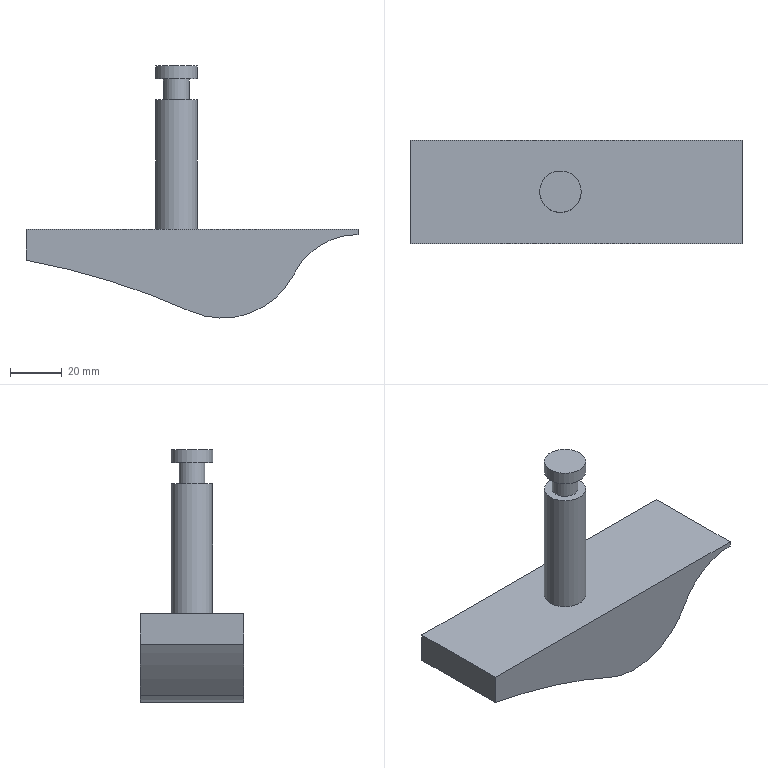Part | STEP file | tieqianhuakuai | 1 solid | 14 faces | box 128 x 40 x 97.212 mm | volume 118551 mm3 | plane 8 | cylinder 6 | commonest cylinder face diameters 16 x2 10 x1 55.183 x1 61.631 x1 558.782 x1
STEP:
#1=CARTESIAN_POINT('',(0.,0.,0.));
#2=DIRECTION('',(0.,0.,1.));
#3=DIRECTION('',(1.,0.,0.));
#4=AXIS2_PLACEMENT_3D('',#1,#2,#3);
#5=CARTESIAN_POINT('',(-8.116,0.,60.7));
#6=VERTEX_POINT('',#5);
#7=CARTESIAN_POINT('',(1.884,0.,60.7));
#8=VERTEX_POINT('',#7);
#9=CARTESIAN_POINT('',(-3.116,0.,60.7));
#10=DIRECTION('',(0.,0.,1.));
#11=DIRECTION('',(1.,0.,0.));
#12=AXIS2_PLACEMENT_3D('',#9,#10,#11);
#13=CIRCLE('',#12,5.);
#14=CARTESIAN_POINT('',(-3.116,0.,60.7));
#15=DIRECTION('',(0.,0.,-1.));
#16=DIRECTION('',(-1.,0.,0.));
#17=AXIS2_PLACEMENT_3D('',#14,#15,#16);
#18=CYLINDRICAL_SURFACE('',#17,5.);
#19=CARTESIAN_POINT('',(9.425,0.));
#20=DIRECTION('',(-1.,0.));
#21=VECTOR('',#20,1.);
#22=LINE('',#19,#21);
#23=(GEOMETRIC_REPRESENTATION_CONTEXT(2)PARAMETRIC_REPRESENTATION_CONTEXT()REPRESENTATION_CONTEXT('',''));
#24=DEFINITIONAL_REPRESENTATION('',(#22),#23);
#25=PCURVE('',#18,#24);
#26=CARTESIAN_POINT('',(-3.116,0.,60.7));
#27=DIRECTION('',(0.,0.,1.));
#28=DIRECTION('',(1.,0.,0.));
#29=AXIS2_PLACEMENT_3D('',#26,#27,#28);
#30=PLANE('',#29);
#31=CARTESIAN_POINT('',(0.,0.));
#32=DIRECTION('',(1.,0.));
#33=AXIS2_PLACEMENT_2D('',#31,#32);
#34=CIRCLE('',#33,5.);
#35=(GEOMETRIC_REPRESENTATION_CONTEXT(2)PARAMETRIC_REPRESENTATION_CONTEXT()REPRESENTATION_CONTEXT('',''));
#36=DEFINITIONAL_REPRESENTATION('',(#34),#35);
#37=PCURVE('',#30,#36);
#38=SURFACE_CURVE('',#13,(#25,#37),.PCURVE_S1.);
#39=EDGE_CURVE('',#6,#8,#38,.T.);
#40=ORIENTED_EDGE('',*,*,#39,.F.);
#41=CARTESIAN_POINT('',(-8.116,0.,52.7));
#42=VERTEX_POINT('',#41);
#43=CARTESIAN_POINT('',(-8.116,0.,60.7));
#44=CARTESIAN_POINT('',(-8.116,0.,52.7));
#45=B_SPLINE_CURVE_WITH_KNOTS('',1,(#43,#44),.UNSPECIFIED.,.F.,.F.,(2,2),(0.,8.),.PIECEWISE_BEZIER_KNOTS.);
#46=CARTESIAN_POINT('',(6.283,0.));
#47=DIRECTION('',(0.,1.));
#48=VECTOR('',#47,1.);
#49=LINE('',#46,#48);
#50=(GEOMETRIC_REPRESENTATION_CONTEXT(2)PARAMETRIC_REPRESENTATION_CONTEXT()REPRESENTATION_CONTEXT('',''));
#51=DEFINITIONAL_REPRESENTATION('',(#49),#50);
#52=PCURVE('',#18,#51);
#53=CARTESIAN_POINT('',(0.,0.));
#54=DIRECTION('',(0.,1.));
#55=VECTOR('',#54,1.);
#56=LINE('',#53,#55);
#57=(GEOMETRIC_REPRESENTATION_CONTEXT(2)PARAMETRIC_REPRESENTATION_CONTEXT()REPRESENTATION_CONTEXT('',''));
#58=DEFINITIONAL_REPRESENTATION('',(#56),#57);
#59=PCURVE('',#18,#58);
#60=SEAM_CURVE('',#45,(#52,#59),.PCURVE_S1.);
#61=EDGE_CURVE('',#6,#42,#60,.T.);
#62=ORIENTED_EDGE('',*,*,#61,.T.);
#63=CARTESIAN_POINT('',(-3.116,0.,52.7));
#64=DIRECTION('',(0.,0.,-1.));
#65=DIRECTION('',(-1.,0.,0.));
#66=AXIS2_PLACEMENT_3D('',#63,#64,#65);
#67=CIRCLE('',#66,5.);
#68=CARTESIAN_POINT('',(0.,8.));
#69=DIRECTION('',(1.,0.));
#70=VECTOR('',#69,1.);
#71=LINE('',#68,#70);
#72=(GEOMETRIC_REPRESENTATION_CONTEXT(2)PARAMETRIC_REPRESENTATION_CONTEXT()REPRESENTATION_CONTEXT('',''));
#73=DEFINITIONAL_REPRESENTATION('',(#71),#72);
#74=PCURVE('',#18,#73);
#75=CARTESIAN_POINT('',(-3.116,0.,52.7));
#76=DIRECTION('',(0.,0.,-1.));
#77=DIRECTION('',(-1.,0.,0.));
#78=AXIS2_PLACEMENT_3D('',#75,#76,#77);
#79=PLANE('',#78);
#80=CARTESIAN_POINT('',(0.,0.));
#81=DIRECTION('',(1.,0.));
#82=AXIS2_PLACEMENT_2D('',#80,#81);
#83=CIRCLE('',#82,5.);
#84=(GEOMETRIC_REPRESENTATION_CONTEXT(2)PARAMETRIC_REPRESENTATION_CONTEXT()REPRESENTATION_CONTEXT('',''));
#85=DEFINITIONAL_REPRESENTATION('',(#83),#84);
#86=PCURVE('',#79,#85);
#87=SURFACE_CURVE('',#67,(#74,#86),.PCURVE_S1.);
#88=EDGE_CURVE('',#42,#42,#87,.T.);
#89=ORIENTED_EDGE('',*,*,#88,.F.);
#90=ORIENTED_EDGE('',*,*,#61,.F.);
#91=CARTESIAN_POINT('',(-3.116,0.,60.7));
#92=DIRECTION('',(0.,0.,1.));
#93=DIRECTION('',(1.,0.,0.));
#94=AXIS2_PLACEMENT_3D('',#91,#92,#93);
#95=CIRCLE('',#94,5.);
#96=CARTESIAN_POINT('',(3.142,0.));
#97=DIRECTION('',(-1.,0.));
#98=VECTOR('',#97,1.);
#99=LINE('',#96,#98);
#100=(GEOMETRIC_REPRESENTATION_CONTEXT(2)PARAMETRIC_REPRESENTATION_CONTEXT()REPRESENTATION_CONTEXT('',''));
#101=DEFINITIONAL_REPRESENTATION('',(#99),#100);
#102=PCURVE('',#18,#101);
#103=CARTESIAN_POINT('',(0.,0.));
#104=DIRECTION('',(1.,0.));
#105=AXIS2_PLACEMENT_2D('',#103,#104);
#106=CIRCLE('',#105,5.);
#107=(GEOMETRIC_REPRESENTATION_CONTEXT(2)PARAMETRIC_REPRESENTATION_CONTEXT()REPRESENTATION_CONTEXT('',''));
#108=DEFINITIONAL_REPRESENTATION('',(#106),#107);
#109=PCURVE('',#30,#108);
#110=SURFACE_CURVE('',#95,(#102,#109),.PCURVE_S1.);
#111=EDGE_CURVE('',#8,#6,#110,.T.);
#112=ORIENTED_EDGE('',*,*,#111,.F.);
#113=EDGE_LOOP('',(#40,#62,#89,#90,#112));
#114=FACE_BOUND('',#113,.T.);
#115=ADVANCED_FACE('',(#114),#18,.T.);
#116=CARTESIAN_POINT('',(4.884,0.,60.7));
#117=VERTEX_POINT('',#116);
#118=CARTESIAN_POINT('',(-3.116,0.,60.7));
#119=DIRECTION('',(0.,0.,1.));
#120=DIRECTION('',(1.,0.,0.));
#121=AXIS2_PLACEMENT_3D('',#118,#119,#120);
#122=CIRCLE('',#121,8.);
#123=CARTESIAN_POINT('',(0.,0.));
#124=DIRECTION('',(1.,0.));
#125=AXIS2_PLACEMENT_2D('',#123,#124);
#126=CIRCLE('',#125,8.);
#127=(GEOMETRIC_REPRESENTATION_CONTEXT(2)PARAMETRIC_REPRESENTATION_CONTEXT()REPRESENTATION_CONTEXT('',''));
#128=DEFINITIONAL_REPRESENTATION('',(#126),#127);
#129=PCURVE('',#30,#128);
#130=CARTESIAN_POINT('',(-3.116,0.,65.7));
#131=DIRECTION('',(0.,0.,-1.));
#132=DIRECTION('',(-1.,0.,0.));
#133=AXIS2_PLACEMENT_3D('',#130,#131,#132);
#134=CYLINDRICAL_SURFACE('',#133,8.);
#135=CARTESIAN_POINT('',(9.425,5.));
#136=DIRECTION('',(-1.,0.));
#137=VECTOR('',#136,1.);
#138=LINE('',#135,#137);
#139=(GEOMETRIC_REPRESENTATION_CONTEXT(2)PARAMETRIC_REPRESENTATION_CONTEXT()REPRESENTATION_CONTEXT('',''));
#140=DEFINITIONAL_REPRESENTATION('',(#138),#139);
#141=PCURVE('',#134,#140);
#142=SURFACE_CURVE('',#122,(#129,#141),.PCURVE_S1.);
#143=EDGE_CURVE('',#117,#117,#142,.T.);
#144=ORIENTED_EDGE('',*,*,#143,.F.);
#145=EDGE_LOOP('',(#144));
#146=FACE_BOUND('',#145,.T.);
#147=ORIENTED_EDGE('',*,*,#111,.T.);
#148=ORIENTED_EDGE('',*,*,#39,.T.);
#149=EDGE_LOOP('',(#147,#148));
#150=FACE_BOUND('',#149,.T.);
#151=ADVANCED_FACE('',(#146,#150),#30,.F.);
#152=CARTESIAN_POINT('',(4.884,0.,65.7));
#153=VERTEX_POINT('',#152);
#154=CARTESIAN_POINT('',(-3.116,0.,65.7));
#155=DIRECTION('',(0.,0.,1.));
#156=DIRECTION('',(1.,0.,0.));
#157=AXIS2_PLACEMENT_3D('',#154,#155,#156);
#158=CIRCLE('',#157,8.);
#159=CARTESIAN_POINT('',(9.425,0.));
#160=DIRECTION('',(-1.,0.));
#161=VECTOR('',#160,1.);
#162=LINE('',#159,#161);
#163=(GEOMETRIC_REPRESENTATION_CONTEXT(2)PARAMETRIC_REPRESENTATION_CONTEXT()REPRESENTATION_CONTEXT('',''));
#164=DEFINITIONAL_REPRESENTATION('',(#162),#163);
#165=PCURVE('',#134,#164);
#166=CARTESIAN_POINT('',(-3.116,0.,65.7));
#167=DIRECTION('',(0.,0.,1.));
#168=DIRECTION('',(1.,0.,0.));
#169=AXIS2_PLACEMENT_3D('',#166,#167,#168);
#170=PLANE('',#169);
#171=CARTESIAN_POINT('',(0.,0.));
#172=DIRECTION('',(1.,0.));
#173=AXIS2_PLACEMENT_2D('',#171,#172);
#174=CIRCLE('',#173,8.);
#175=(GEOMETRIC_REPRESENTATION_CONTEXT(2)PARAMETRIC_REPRESENTATION_CONTEXT()REPRESENTATION_CONTEXT('',''));
#176=DEFINITIONAL_REPRESENTATION('',(#174),#175);
#177=PCURVE('',#170,#176);
#178=SURFACE_CURVE('',#158,(#165,#177),.PCURVE_S1.);
#179=EDGE_CURVE('',#153,#153,#178,.T.);
#180=ORIENTED_EDGE('',*,*,#179,.F.);
#181=CARTESIAN_POINT('',(4.884,0.,65.7));
#182=CARTESIAN_POINT('',(4.884,0.,60.7));
#183=B_SPLINE_CURVE_WITH_KNOTS('',1,(#181,#182),.UNSPECIFIED.,.F.,.F.,(2,2),(0.,5.),.PIECEWISE_BEZIER_KNOTS.);
#184=CARTESIAN_POINT('',(9.425,0.));
#185=DIRECTION('',(0.,1.));
#186=VECTOR('',#185,1.);
#187=LINE('',#184,#186);
#188=(GEOMETRIC_REPRESENTATION_CONTEXT(2)PARAMETRIC_REPRESENTATION_CONTEXT()REPRESENTATION_CONTEXT('',''));
#189=DEFINITIONAL_REPRESENTATION('',(#187),#188);
#190=PCURVE('',#134,#189);
#191=CARTESIAN_POINT('',(3.142,0.));
#192=DIRECTION('',(0.,1.));
#193=VECTOR('',#192,1.);
#194=LINE('',#191,#193);
#195=(GEOMETRIC_REPRESENTATION_CONTEXT(2)PARAMETRIC_REPRESENTATION_CONTEXT()REPRESENTATION_CONTEXT('',''));
#196=DEFINITIONAL_REPRESENTATION('',(#194),#195);
#197=PCURVE('',#134,#196);
#198=SEAM_CURVE('',#183,(#190,#197),.PCURVE_S1.);
#199=EDGE_CURVE('',#153,#117,#198,.T.);
#200=ORIENTED_EDGE('',*,*,#199,.T.);
#201=ORIENTED_EDGE('',*,*,#143,.T.);
#202=ORIENTED_EDGE('',*,*,#199,.F.);
#203=EDGE_LOOP('',(#180,#200,#201,#202));
#204=FACE_BOUND('',#203,.T.);
#205=ADVANCED_FACE('',(#204),#134,.T.);
#206=ORIENTED_EDGE('',*,*,#179,.T.);
#207=EDGE_LOOP('',(#206));
#208=FACE_BOUND('',#207,.T.);
#209=ADVANCED_FACE('',(#208),#170,.T.);
#210=CARTESIAN_POINT('',(-11.116,0.,52.7));
#211=VERTEX_POINT('',#210);
#212=CARTESIAN_POINT('',(-3.116,0.,52.7));
#213=DIRECTION('',(0.,0.,-1.));
#214=DIRECTION('',(-1.,0.,0.));
#215=AXIS2_PLACEMENT_3D('',#212,#213,#214);
#216=CIRCLE('',#215,8.);
#217=CARTESIAN_POINT('',(0.,0.));
#218=DIRECTION('',(1.,0.));
#219=AXIS2_PLACEMENT_2D('',#217,#218);
#220=CIRCLE('',#219,8.);
#221=(GEOMETRIC_REPRESENTATION_CONTEXT(2)PARAMETRIC_REPRESENTATION_CONTEXT()REPRESENTATION_CONTEXT('',''));
#222=DEFINITIONAL_REPRESENTATION('',(#220),#221);
#223=PCURVE('',#79,#222);
#224=CARTESIAN_POINT('',(-3.116,0.,2.7));
#225=DIRECTION('',(0.,0.,1.));
#226=DIRECTION('',(1.,0.,0.));
#227=AXIS2_PLACEMENT_3D('',#224,#225,#226);
#228=CYLINDRICAL_SURFACE('',#227,8.);
#229=CARTESIAN_POINT('',(9.425,50.));
#230=DIRECTION('',(-1.,0.));
#231=VECTOR('',#230,1.);
#232=LINE('',#229,#231);
#233=(GEOMETRIC_REPRESENTATION_CONTEXT(2)PARAMETRIC_REPRESENTATION_CONTEXT()REPRESENTATION_CONTEXT('',''));
#234=DEFINITIONAL_REPRESENTATION('',(#232),#233);
#235=PCURVE('',#228,#234);
#236=SURFACE_CURVE('',#216,(#223,#235),.PCURVE_S1.);
#237=EDGE_CURVE('',#211,#211,#236,.T.);
#238=ORIENTED_EDGE('',*,*,#237,.F.);
#239=EDGE_LOOP('',(#238));
#240=FACE_BOUND('',#239,.T.);
#241=ORIENTED_EDGE('',*,*,#88,.T.);
#242=EDGE_LOOP('',(#241));
#243=FACE_BOUND('',#242,.T.);
#244=ADVANCED_FACE('',(#240,#243),#79,.F.);
#245=CARTESIAN_POINT('',(-11.116,0.,2.7));
#246=VERTEX_POINT('',#245);
#247=CARTESIAN_POINT('',(-3.116,0.,2.7));
#248=DIRECTION('',(0.,0.,-1.));
#249=DIRECTION('',(-1.,0.,0.));
#250=AXIS2_PLACEMENT_3D('',#247,#248,#249);
#251=CIRCLE('',#250,8.);
#252=CARTESIAN_POINT('',(9.425,0.));
#253=DIRECTION('',(-1.,0.));
#254=VECTOR('',#253,1.);
#255=LINE('',#252,#254);
#256=(GEOMETRIC_REPRESENTATION_CONTEXT(2)PARAMETRIC_REPRESENTATION_CONTEXT()REPRESENTATION_CONTEXT('',''));
#257=DEFINITIONAL_REPRESENTATION('',(#255),#256);
#258=PCURVE('',#228,#257);
#259=CARTESIAN_POINT('',(-61.116,-20.,2.7));
#260=DIRECTION('',(0.,0.,1.));
#261=DIRECTION('',(1.,0.,0.));
#262=AXIS2_PLACEMENT_3D('',#259,#260,#261);
#263=PLANE('',#262);
#264=CARTESIAN_POINT('',(50.,20.));
#265=CARTESIAN_POINT('',(50.,33.856));
#266=CARTESIAN_POINT('',(62.,26.928));
#267=CARTESIAN_POINT('',(74.,20.));
#268=CARTESIAN_POINT('',(62.,13.072));
#269=CARTESIAN_POINT('',(50.,6.144));
#270=CARTESIAN_POINT('',(50.,20.));
#271=(BOUNDED_CURVE()B_SPLINE_CURVE(2,(#264,#265,#266,#267,#268,#269,#270),.UNSPECIFIED.,.T.,.F.)B_SPLINE_CURVE_WITH_KNOTS((1,2,2,2,2,1),(-2.094,0.,2.094,4.189,6.283,8.378),.UNSPECIFIED.)CURVE()GEOMETRIC_REPRESENTATION_ITEM()RATIONAL_B_SPLINE_CURVE((1.,0.5,1.,0.5,1.,0.5,1.))REPRESENTATION_ITEM(''));
#272=(GEOMETRIC_REPRESENTATION_CONTEXT(2)PARAMETRIC_REPRESENTATION_CONTEXT()REPRESENTATION_CONTEXT('',''));
#273=DEFINITIONAL_REPRESENTATION('',(#271),#272);
#274=PCURVE('',#263,#273);
#275=SURFACE_CURVE('',#251,(#258,#274),.PCURVE_S1.);
#276=EDGE_CURVE('',#246,#246,#275,.T.);
#277=ORIENTED_EDGE('',*,*,#276,.F.);
#278=CARTESIAN_POINT('',(-11.116,0.,2.7));
#279=CARTESIAN_POINT('',(-11.116,0.,52.7));
#280=B_SPLINE_CURVE_WITH_KNOTS('',1,(#278,#279),.UNSPECIFIED.,.F.,.F.,(2,2),(0.,50.),.PIECEWISE_BEZIER_KNOTS.);
#281=CARTESIAN_POINT('',(9.425,0.));
#282=DIRECTION('',(0.,1.));
#283=VECTOR('',#282,1.);
#284=LINE('',#281,#283);
#285=(GEOMETRIC_REPRESENTATION_CONTEXT(2)PARAMETRIC_REPRESENTATION_CONTEXT()REPRESENTATION_CONTEXT('',''));
#286=DEFINITIONAL_REPRESENTATION('',(#284),#285);
#287=PCURVE('',#228,#286);
#288=CARTESIAN_POINT('',(3.142,0.));
#289=DIRECTION('',(0.,1.));
#290=VECTOR('',#289,1.);
#291=LINE('',#288,#290);
#292=(GEOMETRIC_REPRESENTATION_CONTEXT(2)PARAMETRIC_REPRESENTATION_CONTEXT()REPRESENTATION_CONTEXT('',''));
#293=DEFINITIONAL_REPRESENTATION('',(#291),#292);
#294=PCURVE('',#228,#293);
#295=SEAM_CURVE('',#280,(#287,#294),.PCURVE_S1.);
#296=EDGE_CURVE('',#246,#211,#295,.T.);
#297=ORIENTED_EDGE('',*,*,#296,.T.);
#298=ORIENTED_EDGE('',*,*,#237,.T.);
#299=ORIENTED_EDGE('',*,*,#296,.F.);
#300=EDGE_LOOP('',(#277,#297,#298,#299));
#301=FACE_BOUND('',#300,.T.);
#302=ADVANCED_FACE('',(#301),#228,.T.);
#303=CARTESIAN_POINT('',(66.884,-20.,2.7));
#304=VERTEX_POINT('',#303);
#305=CARTESIAN_POINT('',(66.884,20.,2.7));
#306=VERTEX_POINT('',#305);
#307=CARTESIAN_POINT('',(66.884,-20.,2.7));
#308=DIRECTION('',(0.,1.,0.));
#309=VECTOR('',#308,1.);
#310=LINE('',#307,#309);
#311=CARTESIAN_POINT('',(128.,0.));
#312=DIRECTION('',(0.,1.));
#313=VECTOR('',#312,1.);
#314=LINE('',#311,#313);
#315=(GEOMETRIC_REPRESENTATION_CONTEXT(2)PARAMETRIC_REPRESENTATION_CONTEXT()REPRESENTATION_CONTEXT('',''));
#316=DEFINITIONAL_REPRESENTATION('',(#314),#315);
#317=PCURVE('',#263,#316);
#318=CARTESIAN_POINT('',(66.884,-20.,2.7));
#319=DIRECTION('',(1.,0.,0.));
#320=DIRECTION('',(0.,0.,-1.));
#321=AXIS2_PLACEMENT_3D('',#318,#319,#320);
#322=PLANE('',#321);
#323=CARTESIAN_POINT('',(0.,0.));
#324=DIRECTION('',(0.,1.));
#325=VECTOR('',#324,1.);
#326=LINE('',#323,#325);
#327=(GEOMETRIC_REPRESENTATION_CONTEXT(2)PARAMETRIC_REPRESENTATION_CONTEXT()REPRESENTATION_CONTEXT('',''));
#328=DEFINITIONAL_REPRESENTATION('',(#326),#327);
#329=PCURVE('',#322,#328);
#330=SURFACE_CURVE('',#310,(#317,#329),.PCURVE_S1.);
#331=EDGE_CURVE('',#304,#306,#330,.T.);
#332=ORIENTED_EDGE('',*,*,#331,.T.);
#333=CARTESIAN_POINT('',(-61.116,20.,2.7));
#334=VERTEX_POINT('',#333);
#335=CARTESIAN_POINT('',(-11.116,20.,2.7));
#336=DIRECTION('',(1.,0.,0.));
#337=VECTOR('',#336,1.);
#338=LINE('',#335,#337);
#339=CARTESIAN_POINT('',(50.,40.));
#340=DIRECTION('',(1.,0.));
#341=VECTOR('',#340,1.);
#342=LINE('',#339,#341);
#343=(GEOMETRIC_REPRESENTATION_CONTEXT(2)PARAMETRIC_REPRESENTATION_CONTEXT()REPRESENTATION_CONTEXT('',''));
#344=DEFINITIONAL_REPRESENTATION('',(#342),#343);
#345=PCURVE('',#263,#344);
#346=CARTESIAN_POINT('',(66.884,20.,-26.891));
#347=DIRECTION('',(0.,-1.,0.));
#348=DIRECTION('',(0.,0.,-1.));
#349=AXIS2_PLACEMENT_3D('',#346,#347,#348);
#350=PLANE('',#349);
#351=CARTESIAN_POINT('',(-29.592,-78.));
#352=DIRECTION('',(0.,1.));
#353=VECTOR('',#352,1.);
#354=LINE('',#351,#353);
#355=(GEOMETRIC_REPRESENTATION_CONTEXT(2)PARAMETRIC_REPRESENTATION_CONTEXT()REPRESENTATION_CONTEXT('',''));
#356=DEFINITIONAL_REPRESENTATION('',(#354),#355);
#357=PCURVE('',#350,#356);
#358=SURFACE_CURVE('',#338,(#345,#357),.PCURVE_S1.);
#359=EDGE_CURVE('',#334,#306,#358,.T.);
#360=ORIENTED_EDGE('',*,*,#359,.F.);
#361=CARTESIAN_POINT('',(-61.116,-20.,2.7));
#362=VERTEX_POINT('',#361);
#363=CARTESIAN_POINT('',(-61.116,-20.,2.7));
#364=DIRECTION('',(0.,1.,0.));
#365=VECTOR('',#364,1.);
#366=LINE('',#363,#365);
#367=CARTESIAN_POINT('',(0.,0.));
#368=DIRECTION('',(0.,1.));
#369=VECTOR('',#368,1.);
#370=LINE('',#367,#369);
#371=(GEOMETRIC_REPRESENTATION_CONTEXT(2)PARAMETRIC_REPRESENTATION_CONTEXT()REPRESENTATION_CONTEXT('',''));
#372=DEFINITIONAL_REPRESENTATION('',(#370),#371);
#373=PCURVE('',#263,#372);
#374=CARTESIAN_POINT('',(-61.116,-20.,-9.241));
#375=DIRECTION('',(-1.,0.,0.));
#376=DIRECTION('',(0.,0.,1.));
#377=AXIS2_PLACEMENT_3D('',#374,#375,#376);
#378=PLANE('',#377);
#379=CARTESIAN_POINT('',(11.941,0.));
#380=DIRECTION('',(0.,1.));
#381=VECTOR('',#380,1.);
#382=LINE('',#379,#381);
#383=(GEOMETRIC_REPRESENTATION_CONTEXT(2)PARAMETRIC_REPRESENTATION_CONTEXT()REPRESENTATION_CONTEXT('',''));
#384=DEFINITIONAL_REPRESENTATION('',(#382),#383);
#385=PCURVE('',#378,#384);
#386=SURFACE_CURVE('',#366,(#373,#385),.PCURVE_S1.);
#387=EDGE_CURVE('',#362,#334,#386,.T.);
#388=ORIENTED_EDGE('',*,*,#387,.F.);
#389=CARTESIAN_POINT('',(-11.116,-20.,2.7));
#390=DIRECTION('',(1.,0.,0.));
#391=VECTOR('',#390,1.);
#392=LINE('',#389,#391);
#393=CARTESIAN_POINT('',(50.,0.));
#394=DIRECTION('',(1.,0.));
#395=VECTOR('',#394,1.);
#396=LINE('',#393,#395);
#397=(GEOMETRIC_REPRESENTATION_CONTEXT(2)PARAMETRIC_REPRESENTATION_CONTEXT()REPRESENTATION_CONTEXT('',''));
#398=DEFINITIONAL_REPRESENTATION('',(#396),#397);
#399=PCURVE('',#263,#398);
#400=CARTESIAN_POINT('',(66.884,-20.,-26.891));
#401=DIRECTION('',(0.,-1.,0.));
#402=DIRECTION('',(0.,0.,-1.));
#403=AXIS2_PLACEMENT_3D('',#400,#401,#402);
#404=PLANE('',#403);
#405=CARTESIAN_POINT('',(-29.592,-78.));
#406=DIRECTION('',(0.,1.));
#407=VECTOR('',#406,1.);
#408=LINE('',#405,#407);
#409=(GEOMETRIC_REPRESENTATION_CONTEXT(2)PARAMETRIC_REPRESENTATION_CONTEXT()REPRESENTATION_CONTEXT('',''));
#410=DEFINITIONAL_REPRESENTATION('',(#408),#409);
#411=PCURVE('',#404,#410);
#412=SURFACE_CURVE('',#392,(#399,#411),.PCURVE_S1.);
#413=EDGE_CURVE('',#362,#304,#412,.T.);
#414=ORIENTED_EDGE('',*,*,#413,.T.);
#415=EDGE_LOOP('',(#332,#360,#388,#414));
#416=FACE_BOUND('',#415,.T.);
#417=ORIENTED_EDGE('',*,*,#276,.T.);
#418=EDGE_LOOP('',(#417));
#419=FACE_BOUND('',#418,.T.);
#420=ADVANCED_FACE('',(#416,#419),#263,.T.);
#421=ORIENTED_EDGE('',*,*,#387,.T.);
#422=CARTESIAN_POINT('',(-61.116,20.,-9.241));
#423=VERTEX_POINT('',#422);
#424=CARTESIAN_POINT('',(-61.116,20.,-9.241));
#425=DIRECTION('',(0.,0.,1.));
#426=VECTOR('',#425,1.);
#427=LINE('',#424,#426);
#428=CARTESIAN_POINT('',(0.,40.));
#429=DIRECTION('',(1.,0.));
#430=VECTOR('',#429,1.);
#431=LINE('',#428,#430);
#432=(GEOMETRIC_REPRESENTATION_CONTEXT(2)PARAMETRIC_REPRESENTATION_CONTEXT()REPRESENTATION_CONTEXT('',''));
#433=DEFINITIONAL_REPRESENTATION('',(#431),#432);
#434=PCURVE('',#378,#433);
#435=CARTESIAN_POINT('',(-17.65,-128.));
#436=DIRECTION('',(-1.,0.));
#437=VECTOR('',#436,1.);
#438=LINE('',#435,#437);
#439=(GEOMETRIC_REPRESENTATION_CONTEXT(2)PARAMETRIC_REPRESENTATION_CONTEXT()REPRESENTATION_CONTEXT('',''));
#440=DEFINITIONAL_REPRESENTATION('',(#438),#439);
#441=PCURVE('',#350,#440);
#442=SURFACE_CURVE('',#427,(#434,#441),.PCURVE_S1.);
#443=EDGE_CURVE('',#423,#334,#442,.T.);
#444=ORIENTED_EDGE('',*,*,#443,.F.);
#445=CARTESIAN_POINT('',(-61.116,-20.,-9.241));
#446=VERTEX_POINT('',#445);
#447=CARTESIAN_POINT('',(-61.116,-20.,-9.241));
#448=DIRECTION('',(0.,1.,0.));
#449=VECTOR('',#448,1.);
#450=LINE('',#447,#449);
#451=CARTESIAN_POINT('',(0.,0.));
#452=DIRECTION('',(0.,1.));
#453=VECTOR('',#452,1.);
#454=LINE('',#451,#453);
#455=(GEOMETRIC_REPRESENTATION_CONTEXT(2)PARAMETRIC_REPRESENTATION_CONTEXT()REPRESENTATION_CONTEXT('',''));
#456=DEFINITIONAL_REPRESENTATION('',(#454),#455);
#457=PCURVE('',#378,#456);
#458=CARTESIAN_POINT('',(-111.608,-20.,-284.032));
#459=DIRECTION('',(0.,1.,0.));
#460=DIRECTION('',(0.,0.,1.));
#461=AXIS2_PLACEMENT_3D('',#458,#459,#460);
#462=CYLINDRICAL_SURFACE('',#461,279.391);
#463=CARTESIAN_POINT('',(0.1817,0.));
#464=DIRECTION('',(0.,1.));
#465=VECTOR('',#464,1.);
#466=LINE('',#463,#465);
#467=(GEOMETRIC_REPRESENTATION_CONTEXT(2)PARAMETRIC_REPRESENTATION_CONTEXT()REPRESENTATION_CONTEXT('',''));
#468=DEFINITIONAL_REPRESENTATION('',(#466),#467);
#469=PCURVE('',#462,#468);
#470=SURFACE_CURVE('',#450,(#457,#469),.PCURVE_S1.);
#471=EDGE_CURVE('',#446,#423,#470,.T.);
#472=ORIENTED_EDGE('',*,*,#471,.F.);
#473=CARTESIAN_POINT('',(-61.116,-20.,-9.241));
#474=DIRECTION('',(0.,0.,1.));
#475=VECTOR('',#474,1.);
#476=LINE('',#473,#475);
#477=CARTESIAN_POINT('',(0.,0.));
#478=DIRECTION('',(1.,0.));
#479=VECTOR('',#478,1.);
#480=LINE('',#477,#479);
#481=(GEOMETRIC_REPRESENTATION_CONTEXT(2)PARAMETRIC_REPRESENTATION_CONTEXT()REPRESENTATION_CONTEXT('',''));
#482=DEFINITIONAL_REPRESENTATION('',(#480),#481);
#483=PCURVE('',#378,#482);
#484=CARTESIAN_POINT('',(-17.65,-128.));
#485=DIRECTION('',(-1.,0.));
#486=VECTOR('',#485,1.);
#487=LINE('',#484,#486);
#488=(GEOMETRIC_REPRESENTATION_CONTEXT(2)PARAMETRIC_REPRESENTATION_CONTEXT()REPRESENTATION_CONTEXT('',''));
#489=DEFINITIONAL_REPRESENTATION('',(#487),#488);
#490=PCURVE('',#404,#489);
#491=SURFACE_CURVE('',#476,(#483,#490),.PCURVE_S1.);
#492=EDGE_CURVE('',#446,#362,#491,.T.);
#493=ORIENTED_EDGE('',*,*,#492,.T.);
#494=EDGE_LOOP('',(#421,#444,#472,#493));
#495=FACE_BOUND('',#494,.T.);
#496=ADVANCED_FACE('',(#495),#378,.T.);
#497=CARTESIAN_POINT('',(2.135,-20.,-28.842));
#498=VERTEX_POINT('',#497);
#499=CARTESIAN_POINT('',(-111.608,-20.,-284.032));
#500=DIRECTION('',(0.,-1.,0.));
#501=DIRECTION('',(0.,0.,-1.));
#502=AXIS2_PLACEMENT_3D('',#499,#500,#501);
#503=CIRCLE('',#502,279.391);
#504=CARTESIAN_POINT('',(3.142,0.));
#505=DIRECTION('',(-1.,0.));
#506=VECTOR('',#505,1.);
#507=LINE('',#504,#506);
#508=(GEOMETRIC_REPRESENTATION_CONTEXT(2)PARAMETRIC_REPRESENTATION_CONTEXT()REPRESENTATION_CONTEXT('',''));
#509=DEFINITIONAL_REPRESENTATION('',(#507),#508);
#510=PCURVE('',#462,#509);
#511=CARTESIAN_POINT('',(257.141,-178.492));
#512=DIRECTION('',(1.,0.));
#513=AXIS2_PLACEMENT_2D('',#511,#512);
#514=CIRCLE('',#513,279.391);
#515=(GEOMETRIC_REPRESENTATION_CONTEXT(2)PARAMETRIC_REPRESENTATION_CONTEXT()REPRESENTATION_CONTEXT('',''));
#516=DEFINITIONAL_REPRESENTATION('',(#514),#515);
#517=PCURVE('',#404,#516);
#518=SURFACE_CURVE('',#503,(#510,#517),.PCURVE_S1.);
#519=EDGE_CURVE('',#498,#446,#518,.T.);
#520=ORIENTED_EDGE('',*,*,#519,.F.);
#521=CARTESIAN_POINT('',(2.135,20.,-28.842));
#522=VERTEX_POINT('',#521);
#523=CARTESIAN_POINT('',(2.135,-20.,-28.842));
#524=DIRECTION('',(0.,1.,0.));
#525=VECTOR('',#524,1.);
#526=LINE('',#523,#525);
#527=CARTESIAN_POINT('',(0.4193,0.));
#528=DIRECTION('',(0.,1.));
#529=VECTOR('',#528,1.);
#530=LINE('',#527,#529);
#531=(GEOMETRIC_REPRESENTATION_CONTEXT(2)PARAMETRIC_REPRESENTATION_CONTEXT()REPRESENTATION_CONTEXT('',''));
#532=DEFINITIONAL_REPRESENTATION('',(#530),#531);
#533=PCURVE('',#462,#532);
#534=CARTESIAN_POINT('',(14.68,-20.,-0.6956));
#535=DIRECTION('',(0.,1.,0.));
#536=DIRECTION('',(0.,0.,1.));
#537=AXIS2_PLACEMENT_3D('',#534,#535,#536);
#538=CYLINDRICAL_SURFACE('',#537,30.816);
#539=CARTESIAN_POINT('',(3.561,0.));
#540=DIRECTION('',(0.,1.));
#541=VECTOR('',#540,1.);
#542=LINE('',#539,#541);
#543=(GEOMETRIC_REPRESENTATION_CONTEXT(2)PARAMETRIC_REPRESENTATION_CONTEXT()REPRESENTATION_CONTEXT('',''));
#544=DEFINITIONAL_REPRESENTATION('',(#542),#543);
#545=PCURVE('',#538,#544);
#546=SURFACE_CURVE('',#526,(#533,#545),.PCURVE_S1.);
#547=EDGE_CURVE('',#498,#522,#546,.T.);
#548=ORIENTED_EDGE('',*,*,#547,.T.);
#549=CARTESIAN_POINT('',(-111.608,20.,-284.032));
#550=DIRECTION('',(0.,-1.,0.));
#551=DIRECTION('',(0.,0.,-1.));
#552=AXIS2_PLACEMENT_3D('',#549,#550,#551);
#553=CIRCLE('',#552,279.391);
#554=CARTESIAN_POINT('',(3.142,40.));
#555=DIRECTION('',(-1.,0.));
#556=VECTOR('',#555,1.);
#557=LINE('',#554,#556);
#558=(GEOMETRIC_REPRESENTATION_CONTEXT(2)PARAMETRIC_REPRESENTATION_CONTEXT()REPRESENTATION_CONTEXT('',''));
#559=DEFINITIONAL_REPRESENTATION('',(#557),#558);
#560=PCURVE('',#462,#559);
#561=CARTESIAN_POINT('',(257.141,-178.492));
#562=DIRECTION('',(1.,0.));
#563=AXIS2_PLACEMENT_2D('',#561,#562);
#564=CIRCLE('',#563,279.391);
#565=(GEOMETRIC_REPRESENTATION_CONTEXT(2)PARAMETRIC_REPRESENTATION_CONTEXT()REPRESENTATION_CONTEXT('',''));
#566=DEFINITIONAL_REPRESENTATION('',(#564),#565);
#567=PCURVE('',#350,#566);
#568=SURFACE_CURVE('',#553,(#560,#567),.PCURVE_S1.);
#569=EDGE_CURVE('',#522,#423,#568,.T.);
#570=ORIENTED_EDGE('',*,*,#569,.T.);
#571=ORIENTED_EDGE('',*,*,#471,.F.);
#572=EDGE_LOOP('',(#520,#548,#570,#571));
#573=FACE_BOUND('',#572,.F.);
#574=ADVANCED_FACE('',(#573),#462,.F.);
#575=ORIENTED_EDGE('',*,*,#547,.T.);
#576=CARTESIAN_POINT('',(42.223,20.,-14.516));
#577=VERTEX_POINT('',#576);
#578=CARTESIAN_POINT('',(14.68,20.,-0.6956));
#579=DIRECTION('',(0.,1.,0.));
#580=DIRECTION('',(0.,0.,1.));
#581=AXIS2_PLACEMENT_3D('',#578,#579,#580);
#582=CIRCLE('',#581,30.816);
#583=CARTESIAN_POINT('',(0.,40.));
#584=DIRECTION('',(1.,0.));
#585=VECTOR('',#584,1.);
#586=LINE('',#583,#585);
#587=(GEOMETRIC_REPRESENTATION_CONTEXT(2)PARAMETRIC_REPRESENTATION_CONTEXT()REPRESENTATION_CONTEXT('',''));
#588=DEFINITIONAL_REPRESENTATION('',(#586),#587);
#589=PCURVE('',#538,#588);
#590=CARTESIAN_POINT('',(-57.011,-52.203));
#591=CARTESIAN_POINT('',(-57.011,1.171));
#592=CARTESIAN_POINT('',(-10.788,-25.516));
#593=CARTESIAN_POINT('',(35.436,-52.203));
#594=CARTESIAN_POINT('',(-10.788,-78.891));
#595=CARTESIAN_POINT('',(-57.011,-105.578));
#596=CARTESIAN_POINT('',(-57.011,-52.203));
#597=(BOUNDED_CURVE()B_SPLINE_CURVE(2,(#590,#591,#592,#593,#594,#595,#596),.UNSPECIFIED.,.T.,.F.)B_SPLINE_CURVE_WITH_KNOTS((1,2,2,2,2,1),(-2.094,0.,2.094,4.189,6.283,8.378),.UNSPECIFIED.)CURVE()GEOMETRIC_REPRESENTATION_ITEM()RATIONAL_B_SPLINE_CURVE((1.,0.5,1.,0.5,1.,0.5,1.))REPRESENTATION_ITEM(''));
#598=(GEOMETRIC_REPRESENTATION_CONTEXT(2)PARAMETRIC_REPRESENTATION_CONTEXT()REPRESENTATION_CONTEXT('',''));
#599=DEFINITIONAL_REPRESENTATION('',(#597),#598);
#600=PCURVE('',#350,#599);
#601=SURFACE_CURVE('',#582,(#589,#600),.PCURVE_S1.);
#602=EDGE_CURVE('',#577,#522,#601,.T.);
#603=ORIENTED_EDGE('',*,*,#602,.F.);
#604=CARTESIAN_POINT('',(42.223,-20.,-14.516));
#605=VERTEX_POINT('',#604);
#606=CARTESIAN_POINT('',(42.223,-20.,-14.516));
#607=DIRECTION('',(0.,1.,0.));
#608=VECTOR('',#607,1.);
#609=LINE('',#606,#608);
#610=CARTESIAN_POINT('',(2.036,0.));
#611=DIRECTION('',(0.,1.));
#612=VECTOR('',#611,1.);
#613=LINE('',#610,#612);
#614=(GEOMETRIC_REPRESENTATION_CONTEXT(2)PARAMETRIC_REPRESENTATION_CONTEXT()REPRESENTATION_CONTEXT('',''));
#615=DEFINITIONAL_REPRESENTATION('',(#613),#614);
#616=PCURVE('',#538,#615);
#617=CARTESIAN_POINT('',(66.884,-20.,-26.891));
#618=DIRECTION('',(0.,1.,0.));
#619=DIRECTION('',(0.,0.,1.));
#620=AXIS2_PLACEMENT_3D('',#617,#618,#619);
#621=CYLINDRICAL_SURFACE('',#620,27.592);
#622=CARTESIAN_POINT('',(5.177,0.));
#623=DIRECTION('',(0.,1.));
#624=VECTOR('',#623,1.);
#625=LINE('',#622,#624);
#626=(GEOMETRIC_REPRESENTATION_CONTEXT(2)PARAMETRIC_REPRESENTATION_CONTEXT()REPRESENTATION_CONTEXT('',''));
#627=DEFINITIONAL_REPRESENTATION('',(#625),#626);
#628=PCURVE('',#621,#627);
#629=SURFACE_CURVE('',#609,(#616,#628),.PCURVE_S1.);
#630=EDGE_CURVE('',#605,#577,#629,.T.);
#631=ORIENTED_EDGE('',*,*,#630,.F.);
#632=CARTESIAN_POINT('',(14.68,-20.,-0.6956));
#633=DIRECTION('',(0.,1.,0.));
#634=DIRECTION('',(0.,0.,1.));
#635=AXIS2_PLACEMENT_3D('',#632,#633,#634);
#636=CIRCLE('',#635,30.816);
#637=CARTESIAN_POINT('',(0.,0.));
#638=DIRECTION('',(1.,0.));
#639=VECTOR('',#638,1.);
#640=LINE('',#637,#639);
#641=(GEOMETRIC_REPRESENTATION_CONTEXT(2)PARAMETRIC_REPRESENTATION_CONTEXT()REPRESENTATION_CONTEXT('',''));
#642=DEFINITIONAL_REPRESENTATION('',(#640),#641);
#643=PCURVE('',#538,#642);
#644=CARTESIAN_POINT('',(-57.011,-52.203));
#645=CARTESIAN_POINT('',(-57.011,1.171));
#646=CARTESIAN_POINT('',(-10.788,-25.516));
#647=CARTESIAN_POINT('',(35.436,-52.203));
#648=CARTESIAN_POINT('',(-10.788,-78.891));
#649=CARTESIAN_POINT('',(-57.011,-105.578));
#650=CARTESIAN_POINT('',(-57.011,-52.203));
#651=(BOUNDED_CURVE()B_SPLINE_CURVE(2,(#644,#645,#646,#647,#648,#649,#650),.UNSPECIFIED.,.T.,.F.)B_SPLINE_CURVE_WITH_KNOTS((1,2,2,2,2,1),(-2.094,0.,2.094,4.189,6.283,8.378),.UNSPECIFIED.)CURVE()GEOMETRIC_REPRESENTATION_ITEM()RATIONAL_B_SPLINE_CURVE((1.,0.5,1.,0.5,1.,0.5,1.))REPRESENTATION_ITEM(''));
#652=(GEOMETRIC_REPRESENTATION_CONTEXT(2)PARAMETRIC_REPRESENTATION_CONTEXT()REPRESENTATION_CONTEXT('',''));
#653=DEFINITIONAL_REPRESENTATION('',(#651),#652);
#654=PCURVE('',#404,#653);
#655=SURFACE_CURVE('',#636,(#643,#654),.PCURVE_S1.);
#656=EDGE_CURVE('',#605,#498,#655,.T.);
#657=ORIENTED_EDGE('',*,*,#656,.T.);
#658=EDGE_LOOP('',(#575,#603,#631,#657));
#659=FACE_BOUND('',#658,.T.);
#660=ADVANCED_FACE('',(#659),#538,.T.);
#661=CARTESIAN_POINT('',(66.884,-20.,0.7005));
#662=VERTEX_POINT('',#661);
#663=CARTESIAN_POINT('',(66.884,-20.,-26.891));
#664=DIRECTION('',(0.,-1.,0.));
#665=DIRECTION('',(0.,0.,-1.));
#666=AXIS2_PLACEMENT_3D('',#663,#664,#665);
#667=CIRCLE('',#666,27.592);
#668=CARTESIAN_POINT('',(9.425,0.));
#669=DIRECTION('',(-1.,0.));
#670=VECTOR('',#669,1.);
#671=LINE('',#668,#670);
#672=(GEOMETRIC_REPRESENTATION_CONTEXT(2)PARAMETRIC_REPRESENTATION_CONTEXT()REPRESENTATION_CONTEXT('',''));
#673=DEFINITIONAL_REPRESENTATION('',(#671),#672);
#674=PCURVE('',#621,#673);
#675=CARTESIAN_POINT('',(0.,0.));
#676=DIRECTION('',(1.,0.));
#677=AXIS2_PLACEMENT_2D('',#675,#676);
#678=CIRCLE('',#677,27.592);
#679=(GEOMETRIC_REPRESENTATION_CONTEXT(2)PARAMETRIC_REPRESENTATION_CONTEXT()REPRESENTATION_CONTEXT('',''));
#680=DEFINITIONAL_REPRESENTATION('',(#678),#679);
#681=PCURVE('',#404,#680);
#682=SURFACE_CURVE('',#667,(#674,#681),.PCURVE_S1.);
#683=EDGE_CURVE('',#662,#605,#682,.T.);
#684=ORIENTED_EDGE('',*,*,#683,.F.);
#685=CARTESIAN_POINT('',(66.884,20.,0.7005));
#686=VERTEX_POINT('',#685);
#687=CARTESIAN_POINT('',(66.884,-20.,0.7005));
#688=DIRECTION('',(0.,1.,0.));
#689=VECTOR('',#688,1.);
#690=LINE('',#687,#689);
#691=CARTESIAN_POINT('',(6.283,0.));
#692=DIRECTION('',(0.,1.));
#693=VECTOR('',#692,1.);
#694=LINE('',#691,#693);
#695=(GEOMETRIC_REPRESENTATION_CONTEXT(2)PARAMETRIC_REPRESENTATION_CONTEXT()REPRESENTATION_CONTEXT('',''));
#696=DEFINITIONAL_REPRESENTATION('',(#694),#695);
#697=PCURVE('',#621,#696);
#698=CARTESIAN_POINT('',(2.,0.));
#699=DIRECTION('',(0.,1.));
#700=VECTOR('',#699,1.);
#701=LINE('',#698,#700);
#702=(GEOMETRIC_REPRESENTATION_CONTEXT(2)PARAMETRIC_REPRESENTATION_CONTEXT()REPRESENTATION_CONTEXT('',''));
#703=DEFINITIONAL_REPRESENTATION('',(#701),#702);
#704=PCURVE('',#322,#703);
#705=SURFACE_CURVE('',#690,(#697,#704),.PCURVE_S1.);
#706=EDGE_CURVE('',#662,#686,#705,.T.);
#707=ORIENTED_EDGE('',*,*,#706,.T.);
#708=CARTESIAN_POINT('',(66.884,20.,-26.891));
#709=DIRECTION('',(0.,-1.,0.));
#710=DIRECTION('',(0.,0.,-1.));
#711=AXIS2_PLACEMENT_3D('',#708,#709,#710);
#712=CIRCLE('',#711,27.592);
#713=CARTESIAN_POINT('',(9.425,40.));
#714=DIRECTION('',(-1.,0.));
#715=VECTOR('',#714,1.);
#716=LINE('',#713,#715);
#717=(GEOMETRIC_REPRESENTATION_CONTEXT(2)PARAMETRIC_REPRESENTATION_CONTEXT()REPRESENTATION_CONTEXT('',''));
#718=DEFINITIONAL_REPRESENTATION('',(#716),#717);
#719=PCURVE('',#621,#718);
#720=CARTESIAN_POINT('',(0.,0.));
#721=DIRECTION('',(1.,0.));
#722=AXIS2_PLACEMENT_2D('',#720,#721);
#723=CIRCLE('',#722,27.592);
#724=(GEOMETRIC_REPRESENTATION_CONTEXT(2)PARAMETRIC_REPRESENTATION_CONTEXT()REPRESENTATION_CONTEXT('',''));
#725=DEFINITIONAL_REPRESENTATION('',(#723),#724);
#726=PCURVE('',#350,#725);
#727=SURFACE_CURVE('',#712,(#719,#726),.PCURVE_S1.);
#728=EDGE_CURVE('',#686,#577,#727,.T.);
#729=ORIENTED_EDGE('',*,*,#728,.T.);
#730=ORIENTED_EDGE('',*,*,#630,.F.);
#731=EDGE_LOOP('',(#684,#707,#729,#730));
#732=FACE_BOUND('',#731,.F.);
#733=ADVANCED_FACE('',(#732),#621,.F.);
#734=ORIENTED_EDGE('',*,*,#706,.T.);
#735=CARTESIAN_POINT('',(66.884,20.,2.7));
#736=DIRECTION('',(0.,0.,-1.));
#737=VECTOR('',#736,1.);
#738=LINE('',#735,#737);
#739=CARTESIAN_POINT('',(0.,40.));
#740=DIRECTION('',(1.,0.));
#741=VECTOR('',#740,1.);
#742=LINE('',#739,#741);
#743=(GEOMETRIC_REPRESENTATION_CONTEXT(2)PARAMETRIC_REPRESENTATION_CONTEXT()REPRESENTATION_CONTEXT('',''));
#744=DEFINITIONAL_REPRESENTATION('',(#742),#743);
#745=PCURVE('',#322,#744);
#746=CARTESIAN_POINT('',(-29.592,0.));
#747=DIRECTION('',(1.,0.));
#748=VECTOR('',#747,1.);
#749=LINE('',#746,#748);
#750=(GEOMETRIC_REPRESENTATION_CONTEXT(2)PARAMETRIC_REPRESENTATION_CONTEXT()REPRESENTATION_CONTEXT('',''));
#751=DEFINITIONAL_REPRESENTATION('',(#749),#750);
#752=PCURVE('',#350,#751);
#753=SURFACE_CURVE('',#738,(#745,#752),.PCURVE_S1.);
#754=EDGE_CURVE('',#306,#686,#753,.T.);
#755=ORIENTED_EDGE('',*,*,#754,.F.);
#756=ORIENTED_EDGE('',*,*,#331,.F.);
#757=CARTESIAN_POINT('',(66.884,-20.,2.7));
#758=DIRECTION('',(0.,0.,-1.));
#759=VECTOR('',#758,1.);
#760=LINE('',#757,#759);
#761=CARTESIAN_POINT('',(0.,0.));
#762=DIRECTION('',(1.,0.));
#763=VECTOR('',#762,1.);
#764=LINE('',#761,#763);
#765=(GEOMETRIC_REPRESENTATION_CONTEXT(2)PARAMETRIC_REPRESENTATION_CONTEXT()REPRESENTATION_CONTEXT('',''));
#766=DEFINITIONAL_REPRESENTATION('',(#764),#765);
#767=PCURVE('',#322,#766);
#768=CARTESIAN_POINT('',(-29.592,0.));
#769=DIRECTION('',(1.,0.));
#770=VECTOR('',#769,1.);
#771=LINE('',#768,#770);
#772=(GEOMETRIC_REPRESENTATION_CONTEXT(2)PARAMETRIC_REPRESENTATION_CONTEXT()REPRESENTATION_CONTEXT('',''));
#773=DEFINITIONAL_REPRESENTATION('',(#771),#772);
#774=PCURVE('',#404,#773);
#775=SURFACE_CURVE('',#760,(#767,#774),.PCURVE_S1.);
#776=EDGE_CURVE('',#304,#662,#775,.T.);
#777=ORIENTED_EDGE('',*,*,#776,.T.);
#778=EDGE_LOOP('',(#734,#755,#756,#777));
#779=FACE_BOUND('',#778,.T.);
#780=ADVANCED_FACE('',(#779),#322,.T.);
#781=ORIENTED_EDGE('',*,*,#413,.F.);
#782=ORIENTED_EDGE('',*,*,#492,.F.);
#783=ORIENTED_EDGE('',*,*,#519,.F.);
#784=ORIENTED_EDGE('',*,*,#656,.F.);
#785=ORIENTED_EDGE('',*,*,#683,.F.);
#786=ORIENTED_EDGE('',*,*,#776,.F.);
#787=EDGE_LOOP('',(#781,#782,#783,#784,#785,#786));
#788=FACE_BOUND('',#787,.T.);
#789=ADVANCED_FACE('',(#788),#404,.T.);
#790=ORIENTED_EDGE('',*,*,#359,.T.);
#791=ORIENTED_EDGE('',*,*,#754,.T.);
#792=ORIENTED_EDGE('',*,*,#728,.T.);
#793=ORIENTED_EDGE('',*,*,#602,.T.);
#794=ORIENTED_EDGE('',*,*,#569,.T.);
#795=ORIENTED_EDGE('',*,*,#443,.T.);
#796=EDGE_LOOP('',(#790,#791,#792,#793,#794,#795));
#797=FACE_BOUND('',#796,.T.);
#798=ADVANCED_FACE('',(#797),#350,.F.);
#799=CLOSED_SHELL('',(#115,#151,#205,#209,#244,#302,#420,#496,#574,#660,#733,#780,#789,#798));
#800=MANIFOLD_SOLID_BREP('',#799);
#801=(LENGTH_UNIT()NAMED_UNIT(*)SI_UNIT(.MILLI.,.METRE.));
#802=UNCERTAINTY_MEASURE_WITH_UNIT(LENGTH_MEASURE(0.000002),#801,'','');
#803=(NAMED_UNIT(*)PLANE_ANGLE_UNIT()SI_UNIT($,.RADIAN.));
#804=(NAMED_UNIT(*)SI_UNIT($,.STERADIAN.)SOLID_ANGLE_UNIT());
#805=(GEOMETRIC_REPRESENTATION_CONTEXT(3)GLOBAL_UNCERTAINTY_ASSIGNED_CONTEXT((#802))GLOBAL_UNIT_ASSIGNED_CONTEXT((#801,#803,#804))REPRESENTATION_CONTEXT('',''));
#806=ADVANCED_BREP_SHAPE_REPRESENTATION('',(#4,#800),#805);